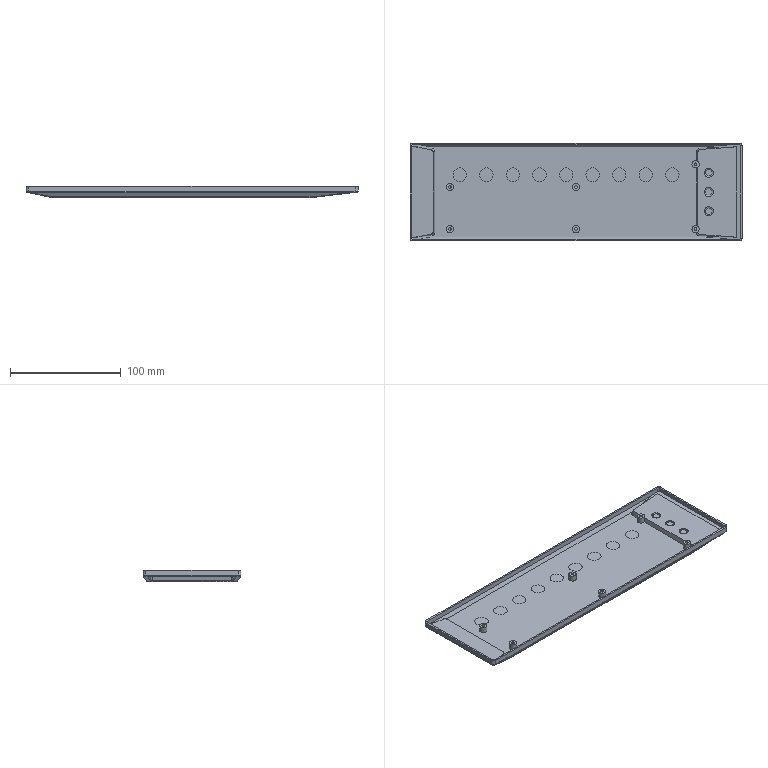NC program | NX | posted with a generic post | part box 300 x 88.5 x 10 mm
Lines 1165 to 2814 of 79950:
(CAVITY_MILL_COPY_COPY_1 , TOOL : D4)
N2322 T04 M6
N2324 G54
N2326 G17 G0 G90 X-96.335 Y33.695 S9500 M3
N2328 G43 Z30. H4
N2330 Z0.8
N2332 G94 G1 Z-0.2 F1000.
N2334 X-96.706 Y34.138
N2336 G3 X-97.473 Y34.495 R1.
N2338 G1 X-98.111 F1650.
N2340 X-98.634 Y34.128
N2342 G3 X-99.055 Y33.396 R1.
N2344 G1 X-99.105 Y32.82
N2346 Z0.8
N2348 G0 X-95.766 Y31.895 Z0.5
N2350 G1 Z-0.5 F1000.
N2352 X-96.138 Y32.338
N2354 G3 X-96.904 Y32.695 R1.
N2356 G1 X-97.542 F1650.
N2358 X-98.065 Y32.328
N2360 G3 X-98.486 Y31.596 R1.
N2362 G1 X-98.536 Y31.02
N2364 Z0.5
N2366 G0 X-95.752 Y31.85 Z0.25
N2368 G1 Z-0.75 F1000.
N2370 X-96.123 Y32.293
N2372 G3 X-96.889 Y32.65 R1.
N2374 G1 X-97.528 F1650.
N2376 X-98.051 Y32.283
N2378 G3 X-98.472 Y31.551 R1.
N2380 G1 X-98.522 Y30.975
N2382 Z0.25
N2384 G0 X-95.752 Y31.85 Z0.
N2386 G1 Z-1. F1000.
N2388 X-96.123 Y32.293
N2390 G3 X-96.889 Y32.65 R1.
N2392 G1 X-97.528 F1650.
N2394 X-98.051 Y32.283
N2396 G3 X-98.472 Y31.551 R1.
N2398 G1 X-98.522 Y30.975
N2400 Z0.
N2402 G0 Z30.
N2404 X-113.253 Y33.33
N2406 Z0.5
N2408 G1 Z-0.5 F1000.
N2410 X-112.81 Y33.702
N2412 G3 X-112.453 Y34.468 R1.
N2414 G1 Y35.999 F1650.
N2416 X-112.732 Y36.02
N2418 G2 X-113.655 Y36.323 R2.
N2420 G3 X-114.493 Y36.429 R1.
N2422 G1 X-114.82 Y36.324
N2424 Z0.5
N2426 G0 X-113.322 Y32.93 Z0.25
N2428 G1 Z-0.75 F1000.
N2430 X-112.879 Y33.302
N2432 G3 X-112.522 Y34.068 R1.
N2434 G1 Y35.935 F1650.
N2436 X-114.384 Y36.07
N2438 G3 X-115.174 Y35.769 R1.
N2440 G1 X-115.518 Y35.414
N2442 Z0.25
N2444 G0 X-113.387 Y32.87 Z0.
N2446 G1 Z-1. F1000.
N2448 X-112.944 Y33.242
N2450 G3 X-112.587 Y34.008 R1.
N2452 G1 Y35.875 F1650.
N2454 X-114.449 Y36.009
N2456 G3 X-115.239 Y35.708 R1.
N2458 G1 X-115.641 Y35.293
N2460 Z0.
N2462 G0 X-113.49 Y32.774 Z-0.378
N2464 G1 Z-1.378 F1000.
N2466 X-113.047 Y33.146
N2468 G3 X-112.69 Y33.912 R1.
N2470 G1 Y35.779 F1650.
N2472 X-114.552 Y35.913
N2474 G3 X-115.342 Y35.612 R1.
N2476 G1 X-115.745 Y35.197
N2478 Z-0.378
N2480 G0 X-113.591 Y32.68 Z-0.756
N2482 G1 Z-1.756 F1000.
N2484 X-113.149 Y33.051
N2486 G3 X-112.791 Y33.817 R1.
N2488 G1 Y35.684 F1650.
N2490 X-114.654 Y35.819
N2492 G3 X-115.443 Y35.518 R1.
N2494 G1 X-115.846 Y35.103
N2496 Z-0.756
N2498 G0 X-113.693 Y32.586 Z-1.133
N2500 G1 Z-2.133 F1000.
N2502 X-113.25 Y32.957
N2504 G3 X-112.893 Y33.723 R1.
N2506 G1 Y35.59 F1650.
N2508 X-114.755 Y35.725
N2510 G3 X-115.545 Y35.424 R1.
N2512 G1 X-115.947 Y35.009
N2514 Z-1.133
N2516 G0 X-113.794 Y32.491 Z-1.511
N2518 G1 Z-2.511 F1000.
N2520 X-113.351 Y32.863
N2522 G3 X-112.994 Y33.629 R1.
N2524 G1 Y35.496 F1650.
N2526 X-114.856 Y35.631
N2528 G3 X-115.646 Y35.33 R1.
N2530 G1 X-116.048 Y34.915
N2532 Z-1.511
N2534 G0 X-113.895 Y32.397 Z-1.889
N2536 G1 Z-2.889 F1000.
N2538 X-113.452 Y32.769
N2540 G3 X-113.095 Y33.535 R1.
N2542 G1 Y35.402 F1650.
N2544 X-114.957 Y35.537
N2546 G3 X-115.747 Y35.236 R1.
N2548 G1 X-116.15 Y34.821
N2550 Z-1.889
N2552 G0 X-113.996 Y32.303 Z-2.267
N2554 G1 Z-3.267 F1000.
N2556 X-113.554 Y32.675
N2558 G3 X-113.196 Y33.441 R1.
N2560 G1 Y35.308 F1650.
N2562 X-115.059 Y35.442
N2564 G3 X-115.848 Y35.141 R1.
N2566 G1 X-116.251 Y34.727
N2568 Z-2.267
N2570 G0 X-114.098 Y32.209 Z-2.644
N2572 G1 Z-3.644 F1000.
N2574 X-113.655 Y32.581
N2576 G3 X-113.298 Y33.347 R1.
N2578 G1 Y35.214 F1650.
N2580 X-115.16 Y35.348
N2582 G3 X-115.95 Y35.047 R1.
N2584 G1 X-116.352 Y34.632
N2586 Z-2.644
N2588 G0 X-114.199 Y32.115 Z-3.022
N2590 G1 Z-4.022 F1000.
N2592 X-113.756 Y32.486
N2594 G3 X-113.399 Y33.252 R1.
N2596 G1 Y35.119 F1650.
N2598 X-115.261 Y35.254
N2600 G3 X-116.051 Y34.953 R1.
N2602 G1 X-116.453 Y34.538
N2604 Z-3.022
N2606 G0 X-114.298 Y32.022 Z-3.4
N2608 G1 Z-4.4 F1000.
N2610 X-113.855 Y32.394
N2612 G3 X-113.498 Y33.16 R1.
N2614 G1 Y35.027 F1650.
N2616 X-115.36 Y35.162
N2618 G3 X-116.15 Y34.861 R1.
N2620 G1 X-116.553 Y34.446
N2622 Z-3.4
N2624 G0 Z30.
N2626 X-100.598 Y31.771
N2628 Z0.8
N2630 G1 Z-0.2 F1000.
N2632 X-101.157 Y31.92
N2634 G3 X-101.989 Y31.772 R1.
N2636 G1 X-102.845 Y31.171 F1650.
N2638 Y30.125
N2640 G3 X-102.488 Y29.359 R1.
N2642 G1 X-102.045 Y28.987
N2644 Z0.8
N2646 G0 X-98.798 Y30.835 Z0.5
N2648 G1 Z-0.5 F1000.
N2650 X-99.357 Y30.984
N2652 G3 X-100.189 Y30.836 R1.
N2654 G1 X-101.045 Y30.235 F1650.
N2656 Y29.189
N2658 G3 X-100.688 Y28.423 R1.
N2660 G1 X-100.245 Y28.052
N2662 Z0.5
N2664 G0 X-98.753 Y30.812 Z0.25
N2666 G1 Z-0.75 F1000.
N2668 X-99.312 Y30.961
N2670 G3 X-100.144 Y30.813 R1.
N2672 G1 X-101. Y30.212 F1650.
N2674 Y29.166
N2676 G3 X-100.643 Y28.4 R1.
N2678 G1 X-100.2 Y28.028
N2680 Z0.25
N2682 G0 X-98.753 Y30.812 Z0.
N2684 G1 Z-1. F1000.
N2686 X-99.312 Y30.961
N2688 G3 X-100.144 Y30.813 R1.
N2690 G1 X-101. Y30.212 F1650.
N2692 Y29.166
N2694 G3 X-100.643 Y28.4 R1.
N2696 G1 X-100.2 Y28.028
N2698 Z0.
N2700 G0 Z30.
N2702 X-118.722 Y18.574
N2704 Z-2.9
N2706 G1 X-118.754 Y18.627 Z-2.903 F1000.
N2708 X-119.176 Y18.964 Z-2.932
N2710 X-119.684 Y19.15 Z-2.96
N2712 X-120.003 Z-2.977
N2714 X-120.319 Z-2.993
N2716 X-120.825 Y18.964 Z-3.021
N2718 X-121.246 Y18.627 Z-3.05
N2720 X-121.574 Y18.086 Z-3.083
N2722 X-121.675 Y17.37 Z-3.121
N2724 X-121.465 Y16.677 Z-3.159
N2726 X-120.983 Y16.138 Z-3.197
N2728 X-120.319 Y15.85 Z-3.235
N2730 X-119.686 Z-3.268
N2732 X-119.02 Y16.135 Z-3.306
N2734 X-118.536 Y16.675 Z-3.344
N2736 X-118.325 Y17.369 Z-3.382
N2738 X-118.426 Y18.086 Z-3.42
N2740 X-118.754 Y18.627 Z-3.453
N2742 X-119.176 Y18.964 Z-3.481
N2744 X-119.684 Y19.15 Z-3.509
N2746 X-120.003 Z-3.526
N2748 X-120.319 Z-3.543
N2750 X-120.825 Y18.964 Z-3.571
N2752 X-121.246 Y18.627 Z-3.599
N2754 X-121.574 Y18.086 Z-3.632
N2756 X-121.675 Y17.37 Z-3.67
N2758 X-121.465 Y16.677 Z-3.708
N2760 X-120.983 Y16.138 Z-3.746
N2762 X-120.319 Y15.85 Z-3.784
N2764 X-119.686 Z-3.817
N2766 X-119.02 Y16.135 Z-3.855
N2768 X-118.536 Y16.675 Z-3.893
N2770 X-118.325 Y17.369 Z-3.931
N2772 X-118.426 Y18.086 Z-3.969
N2774 X-118.754 Y18.627 Z-4.002
N2776 X-119.176 Y18.964 Z-4.031
N2778 X-119.684 Y19.15 Z-4.059
N2780 X-120.003 Z-4.076
N2782 X-120.319 Z-4.092
N2784 X-120.825 Y18.964 Z-4.12
N2786 X-121.246 Y18.627 Z-4.149
N2788 X-121.574 Y18.086 Z-4.182
N2790 X-121.675 Y17.37 Z-4.22
N2792 X-121.465 Y16.677 Z-4.258
N2794 X-120.983 Y16.138 Z-4.296
N2796 X-120.319 Y15.85 Z-4.334
N2798 X-119.686 Z-4.367
N2800 X-119.02 Y16.135 Z-4.405
N2802 X-118.536 Y16.675 Z-4.443
N2804 X-118.325 Y17.369 Z-4.481
N2806 X-118.426 Y18.086 Z-4.519
N2808 X-118.754 Y18.627 Z-4.552
N2810 X-119.176 Y18.964 Z-4.58
N2812 X-119.684 Y19.15 Z-4.608
N2814 X-120. Z-4.625
N2816 X-120.003 F1650.
N2818 G3 X-121.65 Y17.498 R1.65
N2820 X-120. Y19.15 R-1.65
N2822 X-120.766 Y18.793 R1.
N2824 G1 Z-3.625
N2826 G0 Z30.
N2828 X-121.121 Y17.493
N2830 Z-3.125
N2832 G1 X-121.062 Y17.072 Z-3.147 F1000.
N2834 X-120.737 Y16.623 Z-3.176
N2836 X-120.239 Y16.38 Z-3.205
N2838 X-119.718 Y16.39 Z-3.233
N2840 X-119.241 Y16.643 Z-3.261
N2842 X-118.932 Y17.086 Z-3.289
N2844 X-118.861 Y17.621 Z-3.318
N2846 X-119.033 Y18.113 Z-3.345
N2848 X-119.337 Y18.433 Z-3.368
N2850 X-119.74 Y18.615 Z-3.391
N2852 X-120.002 Z-3.405
N2854 X-120.263 Y18.614 Z-3.419
N2856 X-120.664 Y18.433 Z-3.442
N2858 X-120.967 Y18.113 Z-3.465
N2860 X-121.139 Y17.621 Z-3.492
N2862 X-121.062 Y17.072 Z-3.521
N2864 X-120.737 Y16.623 Z-3.55
N2866 X-120.239 Y16.38 Z-3.579
N2868 X-119.718 Y16.39 Z-3.606
N2870 X-119.241 Y16.643 Z-3.635
N2872 X-118.932 Y17.086 Z-3.663
N2874 X-118.861 Y17.621 Z-3.691
N2876 X-119.033 Y18.113 Z-3.719
N2878 X-119.337 Y18.433 Z-3.742
N2880 X-119.74 Y18.615 Z-3.765
N2882 X-120.002 Z-3.779
N2884 X-120.263 Y18.614 Z-3.792
N2886 X-120.664 Y18.433 Z-3.815
N2888 X-120.967 Y18.113 Z-3.839
N2890 X-121.139 Y17.621 Z-3.866
N2892 X-121.062 Y17.072 Z-3.895
N2894 X-120.737 Y16.623 Z-3.924
N2896 X-120.239 Y16.38 Z-3.953
N2898 X-119.718 Y16.39 Z-3.98
N2900 X-119.241 Y16.643 Z-4.009
N2902 X-118.932 Y17.086 Z-4.037
N2904 X-118.861 Y17.621 Z-4.065
N2906 X-119.033 Y18.113 Z-4.092
N2908 X-119.337 Y18.433 Z-4.116
N2910 X-119.74 Y18.615 Z-4.139
N2912 X-120.002 Z-4.153
N2914 X-120.263 Y18.614 Z-4.166
N2916 X-120.664 Y18.433 Z-4.189
N2918 X-120.967 Y18.113 Z-4.212
N2920 X-121.139 Y17.621 Z-4.24
N2922 X-121.062 Y17.072 Z-4.269
N2924 X-120.737 Y16.623 Z-4.298
N2926 X-120.239 Y16.38 Z-4.327
N2928 X-119.718 Y16.39 Z-4.354
N2930 X-119.241 Y16.643 Z-4.382
N2932 X-118.932 Y17.086 Z-4.411
N2934 X-118.861 Y17.621 Z-4.439
N2936 X-119.033 Y18.113 Z-4.466
N2938 X-119.337 Y18.433 Z-4.489
N2940 X-119.74 Y18.615 Z-4.513
N2942 X-120.002 Z-4.526
N2944 X-120.263 Y18.614 Z-4.54
N2946 X-120.664 Y18.433 Z-4.563
N2948 X-120.967 Y18.113 Z-4.586
N2950 X-121.139 Y17.621 Z-4.613
N2952 X-121.062 Y17.072 Z-4.642
N2954 X-120.737 Y16.623 Z-4.672
N2956 X-120.239 Y16.38 Z-4.701
N2958 X-119.718 Y16.39 Z-4.728
N2960 X-119.241 Y16.643 Z-4.756
N2962 X-118.932 Y17.086 Z-4.784
N2964 X-118.861 Y17.621 Z-4.813
N2966 X-119.033 Y18.113 Z-4.84
N2968 X-119.337 Y18.433 Z-4.863
N2970 X-119.74 Y18.615 Z-4.886
N2972 X-120. Z-4.9
N2974 X-120.002 F1650.
N2976 G3 X-121.115 Y17.498 R1.115
N2978 X-120. Y18.615 R-1.115
N2980 X-120.766 Y18.258 R1.
N2982 G1 Z-3.9
N2984 G0 Z30.
N2986 X-121.073 Y1.258
N2988 Z-2.9
N2990 G1 X-121.337 Y1.017 Z-2.919 F1000.
N2992 X-121.618 Y0.451 Z-2.952
N2994 X-121.65 Y0.316 Z-2.959
N2996 Y-0.316 Z-2.992
N2998 X-121.4 Y-0.929 Z-3.027
N3000 X-120.931 Y-1.398 Z-3.062
N3002 X-120.319 Y-1.65 Z-3.096
N3004 X-119.686 Z-3.13
N3006 X-119.049 Y-1.385 Z-3.166
N3008 X-118.573 Y-0.886 Z-3.202
N3010 X-118.337 Y-0.237 Z-3.238
N3012 X-118.382 Y0.451 Z-3.274
N3014 X-118.663 Y1.017 Z-3.307
N3016 X-119.116 Y1.429 Z-3.339
N3018 X-119.686 Y1.65 Z-3.371
N3020 X-120.319 Z-3.405
N3022 X-120.886 Y1.427 Z-3.437
N3024 X-121.337 Y1.017 Z-3.468
N3026 X-121.618 Y0.451 Z-3.502
N3028 X-121.65 Y0.316 Z-3.509
N3030 Y-0.316 Z-3.542
N3032 X-121.4 Y-0.929 Z-3.577
N3034 X-120.931 Y-1.398 Z-3.611
N3036 X-120.319 Y-1.65 Z-3.646
N3038 X-119.686 Z-3.679
N3040 X-119.049 Y-1.385 Z-3.715
N3042 X-118.573 Y-0.886 Z-3.752
N3044 X-118.337 Y-0.237 Z-3.788
N3046 X-118.382 Y0.451 Z-3.824
N3048 X-118.663 Y1.017 Z-3.857
N3050 X-119.116 Y1.429 Z-3.889
N3052 X-119.686 Y1.65 Z-3.921
N3054 X-120.319 Z-3.954
N3056 X-120.886 Y1.427 Z-3.986
N3058 X-121.337 Y1.017 Z-4.018
N3060 X-121.618 Y0.451 Z-4.051
N3062 X-121.65 Y0.316 Z-4.059
N3064 Y-0.316 Z-4.092
N3066 X-121.4 Y-0.929 Z-4.127
N3068 X-120.931 Y-1.398 Z-4.161
N3070 X-120.319 Y-1.65 Z-4.196
N3072 X-119.686 Z-4.229
N3074 X-119.049 Y-1.385 Z-4.265
N3076 X-118.573 Y-0.886 Z-4.301
N3078 X-118.337 Y-0.237 Z-4.338
N3080 X-118.382 Y0.451 Z-4.374
N3082 X-118.663 Y1.017 Z-4.407
N3084 X-119.116 Y1.429 Z-4.439
N3086 X-119.686 Y1.65 Z-4.471
N3088 X-120.319 Z-4.504
N3090 X-120.886 Y1.427 Z-4.536
N3092 X-121.337 Y1.017 Z-4.568
N3094 X-121.618 Y0.451 Z-4.601
N3096 X-121.65 Y0.316 Z-4.608
N3098 Y0. Z-4.625
N3100 G3 X-120. Y-1.65 R1.65 F1650.
N3102 X-121.65 Y0. R-1.65
N3104 X-121.293 Y-0.766 R1.
N3106 G1 Z-3.625
N3108 G0 Z30.
N3110 X-120.024 Y-1.115
N3112 Z-3.125
N3114 G1 X-119.742 Y-1.116 Z-3.14 F1000.
N3116 X-119.287 Y-0.896 Z-3.166
N3118 X-118.971 Y-0.501 Z-3.193
N3120 X-118.855 Y-0.009 Z-3.219
N3122 X-118.969 Y0.499 Z-3.247
N3124 X-119.286 Y0.895 Z-3.273
N3126 X-119.742 Y1.116 Z-3.3
N3128 X-120.263 Y1.114 Z-3.327
N3130 X-120.716 Y0.893 Z-3.353
N3132 X-121.031 Y0.499 Z-3.38
N3134 X-121.115 Y0.124 Z-3.4
N3136 Y-0.26 Z-3.42
N3138 X-120.81 Y-0.809 Z-3.453
N3140 X-120.263 Y-1.114 Z-3.486
N3142 X-119.742 Y-1.116 Z-3.513
N3144 X-119.287 Y-0.896 Z-3.54
N3146 X-118.971 Y-0.501 Z-3.566
N3148 X-118.855 Y-0.009 Z-3.593
N3150 X-118.969 Y0.499 Z-3.62
N3152 X-119.286 Y0.895 Z-3.646
N3154 X-119.742 Y1.116 Z-3.673
N3156 X-120.263 Y1.114 Z-3.7
N3158 X-120.716 Y0.893 Z-3.727
N3160 X-121.031 Y0.499 Z-3.753
N3162 X-121.115 Y0.124 Z-3.773
N3164 Y-0.26 Z-3.793
N3166 X-120.81 Y-0.809 Z-3.826
N3168 X-120.263 Y-1.114 Z-3.859
N3170 X-119.742 Y-1.116 Z-3.887
N3172 X-119.287 Y-0.896 Z-3.913
N3174 X-118.971 Y-0.501 Z-3.94
N3176 X-118.855 Y-0.009 Z-3.966
N3178 X-118.969 Y0.499 Z-3.993
N3180 X-119.286 Y0.895 Z-4.02
N3182 X-119.742 Y1.116 Z-4.046
N3184 X-120.263 Y1.114 Z-4.074
N3186 X-120.716 Y0.893 Z-4.1
N3188 X-121.031 Y0.499 Z-4.127
N3190 X-121.115 Y0.124 Z-4.147
N3192 Y-0.26 Z-4.167
N3194 X-120.81 Y-0.809 Z-4.2
N3196 X-120.263 Y-1.114 Z-4.233
N3198 X-119.742 Y-1.116 Z-4.26
N3200 X-119.287 Y-0.896 Z-4.286
N3202 X-118.971 Y-0.501 Z-4.313
N3204 X-118.855 Y-0.009 Z-4.339
N3206 X-118.969 Y0.499 Z-4.367
N3208 X-119.286 Y0.895 Z-4.393
N3210 X-119.742 Y1.116 Z-4.42
N3212 X-120.263 Y1.114 Z-4.447
N3214 X-120.716 Y0.893 Z-4.474
N3216 X-121.031 Y0.499 Z-4.5
N3218 X-121.115 Y0.124 Z-4.52
N3220 Y-0.26 Z-4.54
N3222 X-120.81 Y-0.809 Z-4.573
N3224 X-120.263 Y-1.114 Z-4.606
N3226 X-119.742 Y-1.116 Z-4.633
N3228 X-119.287 Y-0.896 Z-4.66
N3230 X-118.971 Y-0.501 Z-4.686
N3232 X-118.855 Y-0.009 Z-4.713
N3234 X-118.969 Y0.499 Z-4.74
N3236 X-119.286 Y0.895 Z-4.767
N3238 X-119.742 Y1.116 Z-4.793
N3240 X-120.263 Y1.114 Z-4.82
N3242 X-120.716 Y0.893 Z-4.847
N3244 X-121.031 Y0.499 Z-4.873
N3246 X-121.115 Y0.124 Z-4.894
N3248 Y0. Z-4.9
N3250 G3 X-120. Y-1.115 R1.115 F1650.
N3252 X-121.115 Y0. R-1.115
N3254 X-120.758 Y-0.766 R1.
N3256 G1 Z-3.9
N3258 G0 Z30.
N3260 X-102.045 Y5.626
N3262 Z0.8
N3264 G1 Z-0.2 F1000.
N3266 X-102.488 Y5.255
N3268 G3 X-102.845 Y4.489 R1.
N3270 G1 Y3.507 F1650.
N3272 X-102.071 Y2.902
N3274 G3 X-101.248 Y2.712 R1.
N3276 G1 X-100.682 Y2.833
N3278 Z0.8
N3280 G0 X-100.245 Y6.504 Z0.5
N3282 G1 Z-0.5 F1000.
N3284 X-100.688 Y6.133
N3286 G3 X-101.045 Y5.367 R1.
N3288 G1 Y4.385 F1650.
N3290 X-100.271 Y3.78
N3292 G3 X-99.448 Y3.59 R1.
N3294 G1 X-98.882 Y3.71
N3296 Z0.5
N3298 G0 X-100.2 Y6.526 Z0.25
N3300 G1 Z-0.75 F1000.
N3302 X-100.643 Y6.155
N3304 G3 X-101. Y5.389 R1.
N3306 G1 Y4.407 F1650.
N3308 X-100.226 Y3.802
N3310 G3 X-99.403 Y3.612 R1.
N3312 G1 X-98.837 Y3.732
N3314 Z0.25
N3316 G0 X-100.2 Y6.526 Z0.
N3318 G1 Z-1. F1000.
N3320 X-100.643 Y6.155
N3322 G3 X-101. Y5.389 R1.
N3324 G1 Y4.407 F1650.
N3326 X-100.226 Y3.802
N3328 G3 X-99.403 Y3.612 R1.
N3330 G1 X-98.837 Y3.732
N3332 Z0.
N3334 G0 Z30.
N3336 X-112.898 Y-9.686
N3338 Z0.8
N3340 G1 Z-0.2 F1000.
N3342 X-112.534 Y-9.453
N3344 G3 X-112.081 Y-8.74 R1.
N3346 G2 X-111.655 Y-7.753 R1.953 F1650.
N3348 X-112.058 Y-6.885 R2.04
N3350 G3 X-112.559 Y-6.204 R1.
N3352 G1 X-112.898 Y-6.019
N3354 Z0.8
N3356 G0 Z30.
N3358 Y-19.477
N3360 Z0.8
N3362 G1 Z-0.2 F1000.
N3364 X-112.553 Y-19.29
N3366 G3 X-112.05 Y-18.611 R1.
N3368 G2 X-111.702 Y-17.757 R2.489 F1650.
N3370 X-112.073 Y-16.751 R2.599
N3372 G3 X-112.538 Y-16.045 R1.
N3374 G1 X-112.898 Y-15.823
N3376 Z0.8
N3378 G0 Z30.
N3380 Y-29.706
N3382 Z0.8
N3384 G1 Z-0.2 F1000.
N3386 X-112.539 Y-29.486
N3388 G3 X-112.073 Y-28.781 R1.
N3390 G2 X-111.696 Y-27.701 R3.057 F1650.
N3392 X-112.058 Y-26.885 R2.034
N3394 G3 X-112.559 Y-26.204 R1.
N3396 G1 X-112.898 Y-26.018
N3398 Z0.8
N3400 G0 Z30.
N3402 Y-39.479
N3404 Z0.8
N3406 G1 Z-0.2 F1000.
N3408 X-112.554 Y-39.293
N3410 G3 X-112.052 Y-38.614 R1.
N3412 G2 X-111.688 Y-37.752 R2.371 F1650.
N3414 X-112.074 Y-36.774 R2.318
N3416 G3 X-112.539 Y-36.068 R1.
N3418 G1 X-112.898 Y-35.847
N3420 Z0.8
N3422 G0 X-114.837 Y-36.368 Z0.5
N3424 G1 Z-0.5 F1000.
N3426 X-114.505 Y-36.468
N3428 G3 X-113.669 Y-36.346 R1.
N3430 G2 X-112.662 Y-36.014 R2.038 F1650.
N3432 G1 X-112.453 Y-35.999
N3434 Y-34.468
N3436 G3 X-112.81 Y-33.702 R1.
N3438 G1 X-113.253 Y-33.33
N3440 Z0.5
N3442 G0 X-115.518 Y-35.414 Z0.25
N3444 G1 Z-0.75 F1000.
N3446 X-115.174 Y-35.769
N3448 G3 X-114.384 Y-36.07 R1.
N3450 G1 X-112.522 Y-35.935 F1650.
N3452 Y-34.068
N3454 G3 X-112.879 Y-33.302 R1.
N3456 G1 X-113.322 Y-32.93
N3458 Z0.25
N3460 G0 X-115.641 Y-35.293 Z0.
N3462 G1 Z-1. F1000.
N3464 X-115.239 Y-35.708
N3466 G3 X-114.449 Y-36.009 R1.
N3468 G1 X-112.587 Y-35.875 F1650.
N3470 Y-34.008
N3472 G3 X-112.944 Y-33.242 R1.
N3474 G1 X-113.387 Y-32.87
N3476 Z0.
N3478 G0 X-115.745 Y-35.197 Z-0.378
N3480 G1 Z-1.378 F1000.
N3482 X-115.342 Y-35.612
N3484 G3 X-114.552 Y-35.913 R1.
N3486 G1 X-112.69 Y-35.779 F1650.
N3488 Y-33.912
N3490 G3 X-113.047 Y-33.146 R1.
N3492 G1 X-113.49 Y-32.774
N3494 Z-0.378
N3496 G0 X-115.846 Y-35.103 Z-0.756
N3498 G1 Z-1.756 F1000.
N3500 X-115.443 Y-35.518
N3502 G3 X-114.654 Y-35.819 R1.
N3504 G1 X-112.791 Y-35.684 F1650.
N3506 Y-33.817
N3508 G3 X-113.149 Y-33.051 R1.
N3510 G1 X-113.591 Y-32.68
N3512 Z-0.756
N3514 G0 X-115.947 Y-35.009 Z-1.133
N3516 G1 Z-2.133 F1000.
N3518 X-115.545 Y-35.424
N3520 G3 X-114.755 Y-35.725 R1.
N3522 G1 X-112.893 Y-35.59 F1650.
N3524 Y-33.723
N3526 G3 X-113.25 Y-32.957 R1.
N3528 G1 X-113.693 Y-32.586
N3530 Z-1.133
N3532 G0 X-116.048 Y-34.915 Z-1.511
N3534 G1 Z-2.511 F1000.
N3536 X-115.646 Y-35.33
N3538 G3 X-114.856 Y-35.631 R1.
N3540 G1 X-112.994 Y-35.496 F1650.
N3542 Y-33.629
N3544 G3 X-113.351 Y-32.863 R1.
N3546 G1 X-113.794 Y-32.491
N3548 Z-1.511
N3550 G0 X-116.15 Y-34.821 Z-1.889
N3552 G1 Z-2.889 F1000.
N3554 X-115.747 Y-35.236
N3556 G3 X-114.957 Y-35.537 R1.
N3558 G1 X-113.095 Y-35.402 F1650.
N3560 Y-33.535
N3562 G3 X-113.452 Y-32.769 R1.
N3564 G1 X-113.895 Y-32.397
N3566 Z-1.889
N3568 G0 X-116.251 Y-34.727 Z-2.267
N3570 G1 Z-3.267 F1000.
N3572 X-115.848 Y-35.141
N3574 G3 X-115.059 Y-35.442 R1.
N3576 G1 X-113.196 Y-35.308 F1650.
N3578 Y-33.441
N3580 G3 X-113.554 Y-32.675 R1.
N3582 G1 X-113.996 Y-32.303
N3584 Z-2.267
N3586 G0 X-116.352 Y-34.632 Z-2.644
N3588 G1 Z-3.644 F1000.
N3590 X-115.95 Y-35.047
N3592 G3 X-115.16 Y-35.348 R1.
N3594 G1 X-113.298 Y-35.214 F1650.
N3596 Y-33.347
N3598 G3 X-113.655 Y-32.581 R1.
N3600 G1 X-114.098 Y-32.209
N3602 Z-2.644
N3604 G0 X-116.453 Y-34.538 Z-3.022
N3606 G1 Z-4.022 F1000.
N3608 X-116.051 Y-34.953
N3610 G3 X-115.261 Y-35.254 R1.
N3612 G1 X-113.399 Y-35.119 F1650.
N3614 Y-33.252
N3616 G3 X-113.756 Y-32.486 R1.
N3618 G1 X-114.199 Y-32.115
N3620 Z-3.022
N3622 G0 X-116.553 Y-34.446 Z-3.4
N3624 G1 Z-4.4 F1000.
N3626 X-116.15 Y-34.861
N3628 G3 X-115.36 Y-35.162 R1.
N3630 G1 X-113.498 Y-35.027 F1650.
N3632 Y-33.16
N3634 G3 X-113.855 Y-32.394 R1.
N3636 G1 X-114.298 Y-32.022
N3638 Z-3.4
N3640 G0 Z30.
N3642 X-112.898 Y-34.505
N3644 Z0.8
N3646 G1 Z-0.2 F1000.
N3648 X-112.553 Y-34.313
N3650 G3 X-112.057 Y-33.628 R1.
N3652 G2 X-111.687 Y-32.749 R2.299 F1650.
N3654 X-112.069 Y-31.79 R2.36
N3656 G3 X-112.544 Y-31.091 R1.
N3658 G1 X-112.898 Y-30.879
N3660 Z0.8
N3662 G0 Z30.
N3664 Y-24.346
N3666 Z0.8
N3668 G1 Z-0.2 F1000.
N3670 X-112.569 Y-24.185
N3672 G3 X-112.039 Y-23.526 R1.
N3674 G2 X-111.668 Y-22.762 R2.022 F1650.
N3676 X-112.035 Y-21.984 R2.179
N3678 G3 X-112.565 Y-21.325 R1.
N3680 G1 X-112.898 Y-21.162
N3682 Z0.8
N3684 G0 Z30.
N3686 X-121.292 Y-18.486
N3688 Z-2.9
N3690 G1 X-121.101 Y-18.769 Z-2.918 F1000.
N3692 X-120.319 Y-19.15 Z-2.963
N3694 X-120. Z-2.98
N3696 X-119.684 Z-2.997
N3698 X-118.901 Y-18.77 Z-3.042
N3700 X-118.412 Y-18.05 Z-3.088
N3702 X-118.35 Y-17.181 Z-3.134
N3704 X-118.585 Y-16.594 Z-3.167
N3706 X-119.059 Y-16.108 Z-3.202
N3708 X-119.686 Y-15.85 Z-3.238
N3710 X-120.319 Z-3.271
N3712 X-120.943 Y-16.11 Z-3.306
N3714 X-121.415 Y-16.594 Z-3.342
N3716 X-121.65 Y-17.181 Z-3.375
N3718 X-121.588 Y-18.049 Z-3.421
N3720 X-121.101 Y-18.769 Z-3.466
N3722 X-120.319 Y-19.15 Z-3.512
N3724 X-120. Z-3.528
N3726 X-119.684 Z-3.545
N3728 X-118.901 Y-18.77 Z-3.591
N3730 X-118.412 Y-18.05 Z-3.636
N3732 X-118.35 Y-17.181 Z-3.682
N3734 X-118.585 Y-16.594 Z-3.715
N3736 X-119.059 Y-16.108 Z-3.751
N3738 X-119.686 Y-15.85 Z-3.786
N3740 X-120.319 Z-3.819
N3742 X-120.943 Y-16.11 Z-3.855
N3744 X-121.415 Y-16.594 Z-3.89
N3746 X-121.65 Y-17.181 Z-3.923
N3748 X-121.588 Y-18.049 Z-3.969
N3750 X-121.101 Y-18.769 Z-4.014
N3752 X-120.319 Y-19.15 Z-4.06
N3754 X-120. Z-4.077
N3756 X-119.684 Z-4.093
N3758 X-118.901 Y-18.77 Z-4.139
N3760 X-118.412 Y-18.05 Z-4.185
N3762 X-118.35 Y-17.181 Z-4.23
N3764 X-118.585 Y-16.594 Z-4.263
N3766 X-119.059 Y-16.108 Z-4.299
N3768 X-119.686 Y-15.85 Z-4.334
N3770 X-120.319 Z-4.368
N3772 X-120.943 Y-16.11 Z-4.403
N3774 X-121.415 Y-16.594 Z-4.438
N3776 X-121.65 Y-17.181 Z-4.472
N3778 X-121.588 Y-18.049 Z-4.517
N3780 X-121.101 Y-18.769 Z-4.563
N3782 X-120.319 Y-19.15 Z-4.608
N3784 X-120. Z-4.625
N3786 G3 X-118.35 Y-17.5 R1.65 F1650.
N3788 X-120. Y-19.15 R-1.65
N3790 X-119.234 Y-18.793 R1.
N3792 G1 Z-3.625
N3794 G0 Z30.
N3796 X-118.875 Y-17.565
N3798 Z-3.125
N3800 G1 X-118.925 Y-17.105 Z-3.149 F1000.
N3802 X-119.211 Y-16.67 Z-3.177
N3804 X-119.761 Y-16.38 Z-3.209
N3806 X-120.282 Y-16.39 Z-3.236
N3808 X-120.789 Y-16.67 Z-3.267
N3810 X-121.075 Y-17.105 Z-3.294
N3812 X-121.133 Y-17.663 Z-3.323
N3814 X-120.92 Y-18.181 Z-3.353
N3816 X-120.487 Y-18.536 Z-3.382
N3818 X-120.119 Y-18.615 Z-3.402
N3820 X-120. Z-3.408
N3822 X-119.869 Z-3.415
N3824 X-119.489 Y-18.525 Z-3.435
N3826 X-119.069 Y-18.167 Z-3.464
N3828 X-118.865 Y-17.654 Z-3.493
N3830 X-118.925 Y-17.105 Z-3.522
N3832 X-119.211 Y-16.67 Z-3.55
N3834 X-119.761 Y-16.38 Z-3.582
N3836 X-120.282 Y-16.39 Z-3.609
N3838 X-120.789 Y-16.67 Z-3.64
N3840 X-121.075 Y-17.105 Z-3.667
N3842 X-121.133 Y-17.663 Z-3.696
N3844 X-120.92 Y-18.181 Z-3.726
N3846 X-120.487 Y-18.536 Z-3.755
N3848 X-120.119 Y-18.615 Z-3.775
N3850 X-120. Z-3.781
N3852 X-119.869 Z-3.788
N3854 X-119.489 Y-18.525 Z-3.808
N3856 X-119.069 Y-18.167 Z-3.837
N3858 X-118.865 Y-17.654 Z-3.866
N3860 X-118.925 Y-17.105 Z-3.895
N3862 X-119.211 Y-16.67 Z-3.922
N3864 X-119.761 Y-16.38 Z-3.955
N3866 X-120.282 Y-16.39 Z-3.982
N3868 X-120.789 Y-16.67 Z-4.013
N3870 X-121.075 Y-17.105 Z-4.04
N3872 X-121.133 Y-17.663 Z-4.069
N3874 X-120.92 Y-18.181 Z-4.099
N3876 X-120.487 Y-18.536 Z-4.128
N3878 X-120.119 Y-18.615 Z-4.148
N3880 X-120. Z-4.154
N3882 X-119.869 Z-4.161
N3884 X-119.489 Y-18.525 Z-4.181
N3886 X-119.069 Y-18.167 Z-4.21
N3888 X-118.865 Y-17.654 Z-4.239
N3890 X-118.925 Y-17.105 Z-4.268
N3892 X-119.211 Y-16.67 Z-4.295
N3894 X-119.761 Y-16.38 Z-4.328
N3896 X-120.282 Y-16.39 Z-4.355
N3898 X-120.789 Y-16.67 Z-4.386
N3900 X-121.075 Y-17.105 Z-4.413
N3902 X-121.133 Y-17.663 Z-4.442
N3904 X-120.92 Y-18.181 Z-4.472
N3906 X-120.487 Y-18.536 Z-4.501
N3908 X-120.119 Y-18.615 Z-4.521
N3910 X-120. Z-4.527
N3912 X-119.869 Z-4.534
N3914 X-119.489 Y-18.525 Z-4.554
N3916 X-119.069 Y-18.167 Z-4.583
N3918 X-118.865 Y-17.654 Z-4.612
N3920 X-118.925 Y-17.105 Z-4.641
N3922 X-119.211 Y-16.67 Z-4.668
N3924 X-119.761 Y-16.38 Z-4.701
N3926 X-120.282 Y-16.39 Z-4.728
N3928 X-120.789 Y-16.67 Z-4.759
N3930 X-121.075 Y-17.105 Z-4.786
N3932 X-121.133 Y-17.663 Z-4.815
N3934 X-120.92 Y-18.181 Z-4.845
N3936 X-120.487 Y-18.536 Z-4.874
N3938 X-120.119 Y-18.615 Z-4.894
N3940 X-120. Z-4.9
N3942 G3 X-118.885 Y-17.5 R1.115 F1650.
N3944 X-120. Y-18.615 R-1.115
N3946 X-119.234 Y-18.258 R1.
N3948 G1 Z-3.9
N3950 G0 Z30.
N3952 X-112.898 Y-14.521
N3954 Z0.8
N3956 G1 Z-0.2 F1000.
N3958 X-112.555 Y-14.328
N3960 G3 X-112.063 Y-13.641 R1.
N3962 G2 X-111.683 Y-12.785 R2.041 F1650.
N3964 X-112.066 Y-11.792 R2.644
N3966 G3 X-112.544 Y-11.095 R1.
N3968 G1 X-112.898 Y-10.886
N3970 Z0.8
N3972 G0 Z30.
N3974 X-99.058 Y1.564
N3976 Z0.8
N3978 G1 Z-0.2 F1000.
N3980 X-99.038 Y0.986
N3982 G3 X-98.654 Y0.233 R1.
N3984 G1 X-98.107 Y-0.195 F1650.
N3986 X-97.412
N3988 G3 X-96.646 Y0.162 R1.
N3990 G1 X-96.274 Y0.605
N3992 Z0.8
N3994 G0 X-98.439 Y3.364 Z0.5
N3996 G1 Z-0.5 F1000.
N3998 X-98.418 Y2.786
N4000 G3 X-98.035 Y2.033 R1.
N4002 G1 X-97.487 Y1.605 F1650.
N4004 X-96.792
N4006 G3 X-96.026 Y1.962 R1.
N4008 G1 X-95.654 Y2.405
N4010 Z0.5
N4012 G0 X-98.423 Y3.409 Z0.25
N4014 G1 Z-0.75 F1000.
N4016 X-98.403 Y2.831
N4018 G3 X-98.019 Y2.078 R1.
N4020 G1 X-97.471 Y1.65 F1650.
N4022 X-96.776
N4024 G3 X-96.01 Y2.007 R1.
N4026 G1 X-95.639 Y2.45
N4028 Z0.25
N4030 G0 X-98.423 Y3.409 Z0.
N4032 G1 Z-1. F1000.
N4034 X-98.403 Y2.831
N4036 G3 X-98.019 Y2.078 R1.
N4038 G1 X-97.471 Y1.65 F1650.
N4040 X-96.776
N4042 G3 X-96.01 Y2.007 R1.
N4044 G1 X-95.639 Y2.45
N4046 Z0.
N4048 G0 Z30.
N4050 X-3.856 Y-23.8
N4052 Z0.8
N4054 G1 Z-0.2 F1000.
N4056 X-4.228 Y-23.357
N4058 G3 X-4.994 Y-23. R1.
N4060 G1 X-7. F1650.
N4062 Y-25.006
N4064 G3 X-6.643 Y-25.772 R1.
N4066 G1 X-6.2 Y-26.144
N4068 Z0.8
N4070 G0 X-3.856 Y-23.8 Z0.5
N4072 G1 Z-0.5 F1000.
N4074 X-4.228 Y-23.357
N4076 G3 X-4.994 Y-23. R1.
N4078 G1 X-7. F1650.
N4080 Y-25.006
N4082 G3 X-6.643 Y-25.772 R1.
N4084 G1 X-6.2 Y-26.144
N4086 Z0.5
N4088 G0 Z30.
N4090 Y-29.856
N4092 Z0.8
N4094 G1 Z-0.2 F1000.
N4096 X-6.643 Y-30.228
N4098 G3 X-7. Y-30.994 R1.
N4100 G1 Y-33. F1650.
N4102 X-4.994
N4104 G3 X-4.228 Y-32.643 R1.
N4106 G1 X-3.856 Y-32.2
N4108 Z0.8
N4110 G0 X-6.2 Y-29.856 Z0.5
N4112 G1 Z-0.5 F1000.
N4114 X-6.643 Y-30.228
N4116 G3 X-7. Y-30.994 R1.
N4118 G1 Y-33. F1650.
N4120 X-4.994
N4122 G3 X-4.228 Y-32.643 R1.
N4124 G1 X-3.856 Y-32.2
N4126 Z0.5
N4128 G0 Z30.
N4130 X96.2 Y-26.144
N4132 Z0.8
N4134 G1 Z-0.2 F1000.
N4136 X96.643 Y-25.772
N4138 G3 X97. Y-25.006 R1.
N4140 G1 Y-23. F1650.
N4142 X94.994
N4144 G3 X94.228 Y-23.357 R1.
N4146 G1 X93.856 Y-23.8
N4148 Z0.8
N4150 G0 X96.2 Y-26.144 Z0.5
N4152 G1 Z-0.5 F1000.
N4154 X96.643 Y-25.772
N4156 G3 X97. Y-25.006 R1.
N4158 G1 X96.999 Y-23. F1650.
N4160 X94.994
N4162 G3 X94.228 Y-23.357 R1.
N4164 G1 X93.856 Y-23.8
N4166 Z0.5
N4168 G0 Z30.
N4170 Y-32.2
N4172 Z0.8
N4174 G1 Z-0.2 F1000.
N4176 X94.228 Y-32.643
N4178 G3 X94.994 Y-33. R1.
N4180 G1 X97. F1650.
N4182 Y-30.994
N4184 G3 X96.643 Y-30.228 R1.
N4186 G1 X96.2 Y-29.856
N4188 Z0.8
N4190 G0 X93.856 Y-32.2 Z0.5
N4192 G1 Z-0.5 F1000.
N4194 X94.228 Y-32.643
N4196 G3 X94.994 Y-33. R1.
N4198 G1 X97. F1650.
N4200 Y-30.994
N4202 G3 X96.643 Y-30.228 R1.
N4204 G1 X96.2 Y-29.856
N4206 Z0.5
N4208 G0 Z30.
N4210 X130.205 Y-36.151
N4212 Z0.8
N4214 G1 Z-0.2 F1000.
N4216 X129.875 Y-36.313
N4218 G3 X129.346 Y-36.972 R1.
N4220 G2 X128.965 Y-37.751 R2.042 F1650.
N4222 X129.346 Y-38.525 R2.013
N4224 G3 X129.876 Y-39.183 R1.
N4226 G1 X130.205 Y-39.345
N4228 Z0.8
N4230 G0 Z30.
N4232 X132.201 Y-34.02
N4234 Z0.25
N4236 G1 Z-0.75 F1000.
N4238 X131.759 Y-34.391
N4240 G3 X131.401 Y-35.157 R1.
N4242 G1 Y-35.889 F1650.
N4244 G2 X131.807 Y-36.455 R2.125
N4246 G3 X132.466 Y-36.985 R1.
N4248 G1 X132.807 Y-37.069
N4250 Z0.25
N4252 G0 X132.266 Y-33.407 Z0.
N4254 G1 Z-1. F1000.
N4256 X131.824 Y-33.778
N4258 G3 X131.466 Y-34.545 R1.
N4260 G1 Y-35.833 F1650.
N4262 G2 X132.42 Y-36.256 R2.007
N4264 G3 X133.24 Y-36.46 R1.
N4266 G1 X133.578 Y-36.394
N4268 Z0.
N4270 G0 X132.37 Y-32.925 Z-0.378
N4272 G1 Z-1.378 F1000.
N4274 X131.927 Y-33.297
N4276 G3 X131.57 Y-34.063 R1.
N4278 G1 Y-35.747 F1650.
N4280 X133.229 Y-36.039
N4282 G3 X134.042 Y-35.809 R1.
N4284 G1 X134.306 Y-35.581
N4286 Z-0.378
N4288 G0 X132.471 Y-32.84 Z-0.756
N4290 G1 Z-1.756 F1000.
N4292 X132.028 Y-33.212
N4294 G3 X131.671 Y-33.978 R1.
N4296 G1 Y-35.662 F1650.
N4298 X133.33 Y-35.955
N4300 G3 X134.146 Y-35.736 R1.
N4302 G1 X134.589 Y-35.365
N4304 Z-0.756
N4306 G0 X132.572 Y-32.755 Z-1.133
N4308 G1 Z-2.133 F1000.
N4310 X132.129 Y-33.127
N4312 G3 X131.772 Y-33.893 R1.
N4314 G1 Y-35.577 F1650.
N4316 X133.431 Y-35.87
N4318 G3 X134.248 Y-35.651 R1.
N4320 G1 X134.69 Y-35.28
N4322 Z-1.133
N4324 G0 X132.673 Y-32.67 Z-1.511
N4326 G1 Z-2.511 F1000.
N4328 X132.231 Y-33.042
N4330 G3 X131.873 Y-33.808 R1.
N4332 G1 Y-35.492 F1650.
N4334 X133.532 Y-35.785
N4336 G3 X134.349 Y-35.566 R1.
N4338 G1 X134.792 Y-35.195
N4340 Z-1.511
N4342 G0 X132.775 Y-32.585 Z-1.889
N4344 G1 Z-2.889 F1000.
N4346 X132.332 Y-32.957
N4348 G3 X131.975 Y-33.723 R1.
N4350 G1 Y-35.408 F1650.
N4352 X133.634 Y-35.7
N4354 G3 X134.45 Y-35.481 R1.
N4356 G1 X134.893 Y-35.11
N4358 Z-1.889
N4360 G0 X132.876 Y-32.5 Z-2.267
N4362 G1 Z-3.267 F1000.
N4364 X132.433 Y-32.872
N4366 G3 X132.076 Y-33.638 R1.
N4368 G1 Y-35.323 F1650.
N4370 X133.735 Y-35.615
N4372 G3 X134.551 Y-35.396 R1.
N4374 G1 X134.994 Y-35.025
N4376 Z-2.267
N4378 G0 X132.977 Y-32.415 Z-2.644
N4380 G1 Z-3.644 F1000.
N4382 X132.534 Y-32.787
N4384 G3 X132.177 Y-33.553 R1.
N4386 G1 Y-35.238 F1650.
N4388 X133.836 Y-35.53
N4390 G3 X134.652 Y-35.311 R1.
N4392 G1 X135.095 Y-34.94
N4394 Z-2.644
N4396 G0 X133.078 Y-32.33 Z-3.022
N4398 G1 Z-4.022 F1000.
N4400 X132.635 Y-32.702
N4402 G3 X132.278 Y-33.468 R1.
N4404 G1 Y-35.153 F1650.
N4406 X133.937 Y-35.445
N4408 G3 X134.754 Y-35.226 R1.
N4410 G1 X135.196 Y-34.855
N4412 Z-3.022
N4414 G0 X133.177 Y-32.247 Z-3.4
N4416 G1 Z-4.4 F1000.
N4418 X132.735 Y-32.619
N4420 G3 X132.377 Y-33.385 R1.
N4422 G1 Y-35.069 F1650.
N4424 X134.036 Y-35.362
N4426 G3 X134.853 Y-35.143 R1.
N4428 G1 X135.296 Y-34.772
N4430 Z-3.4
N4432 G0 X133.24 Y-32.195 Z-3.625
N4434 G1 Z-4.625 F1000.
N4436 X132.797 Y-32.566
N4438 G3 X132.44 Y-33.333 R1.
N4440 G1 Y-35.017 F1650.
N4442 X134.099 Y-35.31
N4444 G3 X134.915 Y-35.091 R1.
N4446 G1 X135.358 Y-34.719
N4448 Z-3.625
N4450 G0 X133.298 Y-32.146 Z-3.85
N4452 G1 Z-4.85 F1000.
N4454 X132.855 Y-32.518
N4456 G3 X132.498 Y-33.284 R1.
N4458 G1 Y-34.968 F1650.
N4460 X134.157 Y-35.261
N4462 G3 X134.973 Y-35.042 R1.
N4464 G1 X135.416 Y-34.671
N4466 Z-3.85
N4468 G0 Z30.
N4470 X130.205 Y-30.957
N4472 Z0.8
N4474 G1 Z-0.2 F1000.
N4476 X129.855 Y-31.157
N4478 G3 X129.367 Y-31.848 R1.
N4480 G2 X129.02 Y-32.737 R2.482 F1650.
N4482 X129.371 Y-33.698 R2.791
N4484 G3 X129.85 Y-34.394 R1.
N4486 G1 X130.205 Y-34.604
N4488 Z0.8
N4490 G0 Z30.
N4492 Y-26.023
N4494 Z0.8
N4496 G1 Z-0.2 F1000.
N4498 X129.866 Y-26.209
N4500 G3 X129.366 Y-26.89 R1.
N4502 G2 X128.97 Y-27.744 R2.01 F1650.
N4504 X129.363 Y-28.604 R2.091
N4506 G3 X129.866 Y-29.283 R1.
N4508 G1 X130.205 Y-29.468
N4510 Z0.8
N4512 G0 Z30.
N4514 Y-21.152
N4516 Z0.8
N4518 G1 Z-0.2 F1000.
N4520 X129.877 Y-21.314
N4522 G3 X129.348 Y-21.974 R1.
N4524 G2 X128.965 Y-22.749 R1.984 F1650.
N4526 X129.347 Y-23.525 R2.02
N4528 G3 X129.876 Y-24.184 R1.
N4530 G1 X130.205 Y-24.346
N4532 Z0.8
N4534 G0 Z30.
N4536 Y-16.153
N4538 Z0.8
N4540 G1 Z-0.2 F1000.
N4542 X129.876 Y-16.315
N4544 G3 X129.346 Y-16.973 R1.
N4546 G2 X128.966 Y-17.75 R2.033 F1650.
N4548 X129.346 Y-18.528 R2.047
N4550 G3 X129.875 Y-19.187 R1.
N4552 G1 X130.205 Y-19.349
N4554 Z0.8
N4556 G0 Z30.
N4558 Y-11.141
N4560 Z0.8
N4562 G1 Z-0.2 F1000.
N4564 X129.875 Y-11.305
N4566 G3 X129.348 Y-11.966 R1.
N4568 G2 X128.964 Y-12.752 R2.037 F1650.
N4570 X129.348 Y-13.53 R2.005
N4572 G3 X129.876 Y-14.189 R1.
N4574 G1 X130.205 Y-14.351
N4576 Z0.8
N4578 G0 Z30.
N4580 Y-6.134
N4582 Z0.8
N4584 G1 Z-0.2 F1000.
N4586 X129.874 Y-6.299
N4588 G3 X129.348 Y-6.96 R1.
N4590 G2 X128.965 Y-7.75 R2.056 F1650.
N4592 X129.347 Y-8.531 R2.044
N4594 G3 X129.875 Y-9.191 R1.
N4596 G1 X130.205 Y-9.354
N4598 Z0.8
N4600 G0 Z30.
N4602 X114.7 Y0.605
N4604 Z0.8
N4606 G1 Z-0.2 F1000.
N4608 X115.072 Y0.162
N4610 G3 X115.838 Y-0.195 R1.
N4612 G1 X116.592 F1650.
N4614 X117.161 Y0.3
N4616 G3 X117.505 Y1.072 R1.
N4618 G1 X117.495 Y1.65
N4620 Z0.8
N4622 G0 X114.027 Y2.405 Z0.5
N4624 G1 Z-0.5 F1000.
N4626 X114.399 Y1.962
N4628 G3 X115.165 Y1.605 R1.
N4630 G1 X115.919 F1650.
N4632 X116.488 Y2.1
N4634 G3 X116.832 Y2.872 R1.
N4636 G1 X116.822 Y3.45
N4638 Z0.5
N4640 G0 X114.01 Y2.45 Z0.25
N4642 G1 Z-0.75 F1000.
N4644 X114.382 Y2.007
N4646 G3 X115.148 Y1.65 R1.
N4648 G1 X115.902 F1650.
N4650 X116.471 Y2.145
N4652 G3 X116.815 Y2.917 R1.
N4654 G1 X116.805 Y3.495
N4656 Z0.25
N4658 G0 X114.01 Y2.45 Z0.
N4660 G1 Z-1. F1000.
N4662 X114.382 Y2.007
N4664 G3 X115.148 Y1.65 R1.
N4666 G1 X115.902 F1650.
N4668 X116.471 Y2.145
N4670 G3 X116.815 Y2.917 R1.
N4672 G1 X116.805 Y3.495
N4674 Z0.
N4676 G0 Z30.
N4678 X118.769 Y2.757
N4680 Z0.8
N4682 G1 Z-0.2 F1000.
N4684 X119.34 Y2.667
N4686 G3 X120.152 Y2.9 R1.
N4688 G1 X120.845 Y3.502 F1650.
N4690 Y4.42
N4692 G3 X120.488 Y5.186 R1.
N4694 G1 X120.045 Y5.558
N4696 Z0.8
N4698 G0 X116.969 Y3.578 Z0.5
N4700 G1 Z-0.5 F1000.
N4702 X117.54 Y3.487
N4704 G3 X118.352 Y3.72 R1.
N4706 G1 X119.045 Y4.322 F1650.
N4708 Y5.24
N4710 G3 X118.688 Y6.006 R1.
N4712 G1 X118.245 Y6.378
N4714 Z0.5
N4716 G0 X116.924 Y3.598 Z0.25
N4718 G1 Z-0.75 F1000.
N4720 X117.495 Y3.508
N4722 G3 X118.307 Y3.741 R1.
N4724 G1 X119. Y4.343 F1650.
N4726 Y5.261
N4728 G3 X118.643 Y6.027 R1.
N4730 G1 X118.2 Y6.398
N4732 Z0.25
N4734 G0 X116.924 Y3.598 Z0.
N4736 G1 Z-1. F1000.
N4738 X117.495 Y3.508
N4740 G3 X118.307 Y3.741 R1.
N4742 G1 X119. Y4.343 F1650.
N4744 Y5.261
N4746 G3 X118.643 Y6.027 R1.
N4748 G1 X118.2 Y6.398
N4750 Z0.
N4752 G0 Z30.
N4754 X120.045 Y29.056
N4756 Z0.8
N4758 G1 Z-0.2 F1000.
N4760 X120.488 Y29.428
N4762 G3 X120.845 Y30.194 R1.
N4764 G1 Y31.176 F1650.
N4766 X120.071 Y31.78
N4768 G3 X119.248 Y31.97 R1.
N4770 G1 X118.682 Y31.85
N4772 Z0.8
N4774 G0 X118.245 Y28.178 Z0.5
N4776 G1 Z-0.5 F1000.
N4778 X118.688 Y28.55
N4780 G3 X119.045 Y29.316 R1.
N4782 G1 Y30.298 F1650.
N4784 X118.271 Y30.902
N4786 G3 X117.448 Y31.093 R1.
N4788 G1 X116.882 Y30.972
N4790 Z0.5
N4792 G0 X118.2 Y28.156 Z0.25
N4794 G1 Z-0.75 F1000.
N4796 X118.643 Y28.528
N4798 G3 X119. Y29.294 R1.
N4800 G1 Y30.276 F1650.
N4802 X118.226 Y30.88
N4804 G3 X117.403 Y31.071 R1.
N4806 G1 X116.837 Y30.95
N4808 Z0.25
N4810 G0 X118.2 Y28.156 Z0.
N4812 G1 Z-1. F1000.
N4814 X118.643 Y28.528
N4816 G3 X119. Y29.294 R1.
N4818 G1 Y30.276 F1650.
N4820 X118.226 Y30.88
N4822 G3 X117.403 Y31.071 R1.
N4824 G1 X116.837 Y30.95
N4826 Z0.
N4828 G0 Z30.
N4830 X117.548 Y32.736
N4832 Z0.8
N4834 G1 Z-0.2 F1000.
N4836 X117.528 Y33.314
N4838 G3 X117.144 Y34.067 R1.
N4840 G1 X116.597 Y34.495 F1650.
N4842 X115.902
N4844 G3 X115.135 Y34.138 R1.
N4846 G1 X114.764 Y33.695
N4848 Z0.8
N4850 G0 X116.928 Y30.936 Z0.5
N4852 G1 Z-0.5 F1000.
N4854 X116.908 Y31.514
N4856 G3 X116.525 Y32.267 R1.
N4858 G1 X115.977 Y32.695 F1650.
N4860 X115.282
N4862 G3 X114.516 Y32.338 R1.
N4864 G1 X114.144 Y31.895
N4866 Z0.5
N4868 G0 X116.913 Y30.891 Z0.25
N4870 G1 Z-0.75 F1000.
N4872 X116.893 Y31.469
N4874 G3 X116.509 Y32.222 R1.
N4876 G1 X115.961 Y32.65 F1650.
N4878 X115.266
N4880 G3 X114.5 Y32.293 R1.
N4882 G1 X114.129 Y31.85
N4884 Z0.25
N4886 G0 X116.913 Y30.891 Z0.
N4888 G1 Z-1. F1000.
N4890 X116.893 Y31.469
N4892 G3 X116.509 Y32.222 R1.
N4894 G1 X115.961 Y32.65 F1650.
N4896 X115.266
N4898 G3 X114.5 Y32.293 R1.
N4900 G1 X114.129 Y31.85
N4902 Z0.
N4904 G0 Z30.
N4906 X132.813 Y37.1
N4908 Z0.25
N4910 G1 Z-0.75 F1000.
N4912 X132.479 Y37.016
N4914 G3 X131.822 Y36.484 R1.
N4916 G2 X131.401 Y35.909 R2.008 F1650.
N4918 G1 Y35.158
N4920 G3 X131.759 Y34.391 R1.
N4922 G1 X132.201 Y34.02
N4924 Z0.25
N4926 G0 X133.586 Y36.41 Z0.
N4928 G1 Z-1. F1000.
N4930 X133.248 Y36.474
N4932 G3 X132.429 Y36.265 R1.
N4934 G2 X131.466 Y35.834 R2.007 F1650.
N4936 G1 Y34.539
N4938 G3 X131.824 Y33.773 R1.
N4940 G1 X132.266 Y33.401
N4942 Z0.
N4944 G0 X134.306 Y35.58 Z-0.378
N4946 G1 Z-1.378 F1000.
N4948 X134.042 Y35.808
N4950 G3 X133.229 Y36.039 R1.
N4952 G1 X131.57 Y35.747 F1650.
N4954 Y34.063
N4956 G3 X131.927 Y33.297 R1.
N4958 G1 X132.37 Y32.925
N4960 Z-0.378
N4962 G0 X134.589 Y35.365 Z-0.756
N4964 G1 Z-1.756 F1000.
N4966 X134.146 Y35.736
N4968 G3 X133.33 Y35.955 R1.
N4970 G1 X131.671 Y35.662 F1650.
N4972 Y33.978
N4974 G3 X132.028 Y33.212 R1.
N4976 G1 X132.471 Y32.84
N4978 Z-0.756
N4980 G0 X134.69 Y35.28 Z-1.133
N4982 G1 Z-2.133 F1000.
N4984 X134.248 Y35.651
N4986 G3 X133.431 Y35.87 R1.
N4988 G1 X131.772 Y35.577 F1650.
N4990 Y33.893
N4992 G3 X132.129 Y33.127 R1.
N4994 G1 X132.572 Y32.755
N4996 Z-1.133
N4998 G0 X134.792 Y35.195 Z-1.511
N5000 G1 Z-2.511 F1000.
N5002 X134.349 Y35.566
N5004 G3 X133.532 Y35.785 R1.
N5006 G1 X131.873 Y35.492 F1650.
N5008 Y33.808
N5010 G3 X132.231 Y33.042 R1.
N5012 G1 X132.673 Y32.67
N5014 Z-1.511
N5016 G0 X134.893 Y35.11 Z-1.889
N5018 G1 Z-2.889 F1000.
N5020 X134.45 Y35.481
N5022 G3 X133.634 Y35.7 R1.
N5024 G1 X131.975 Y35.408 F1650.
N5026 Y33.723
N5028 G3 X132.332 Y32.957 R1.
N5030 G1 X132.775 Y32.585
N5032 Z-1.889
N5034 G0 X134.994 Y35.025 Z-2.267
N5036 G1 Z-3.267 F1000.
N5038 X134.551 Y35.396
N5040 G3 X133.735 Y35.615 R1.
N5042 G1 X132.076 Y35.323 F1650.
N5044 Y33.638
N5046 G3 X132.433 Y32.872 R1.
N5048 G1 X132.876 Y32.5
N5050 Z-2.267
N5052 G0 X135.095 Y34.94 Z-2.644
N5054 G1 Z-3.644 F1000.
N5056 X134.652 Y35.311
N5058 G3 X133.836 Y35.53 R1.
N5060 G1 X132.177 Y35.238 F1650.
N5062 Y33.553
N5064 G3 X132.534 Y32.787 R1.
N5066 G1 X132.977 Y32.415
N5068 Z-2.644
N5070 G0 X135.196 Y34.855 Z-3.022
N5072 G1 Z-4.022 F1000.
N5074 X134.754 Y35.226
N5076 G3 X133.937 Y35.445 R1.
N5078 G1 X132.278 Y35.153 F1650.
N5080 Y33.468
N5082 G3 X132.635 Y32.702 R1.
N5084 G1 X133.078 Y32.33
N5086 Z-3.022
N5088 G0 X135.296 Y34.772 Z-3.4
N5090 G1 Z-4.4 F1000.
N5092 X134.853 Y35.143
N5094 G3 X134.036 Y35.362 R1.
N5096 G1 X132.377 Y35.069 F1650.
N5098 Y33.385
N5100 G3 X132.735 Y32.619 R1.
N5102 G1 X133.177 Y32.247
N5104 Z-3.4
N5106 G0 X135.358 Y34.719 Z-3.625
N5108 G1 Z-4.625 F1000.
N5110 X134.915 Y35.091
N5112 G3 X134.099 Y35.31 R1.
N5114 G1 X132.44 Y35.017 F1650.
N5116 Y33.333
N5118 G3 X132.797 Y32.566 R1.
N5120 G1 X133.24 Y32.195
N5122 Z-3.625
N5124 G0 X135.416 Y34.671 Z-3.85
N5126 G1 Z-4.85 F1000.
N5128 X134.973 Y35.042
N5130 G3 X134.157 Y35.261 R1.
N5132 G1 X132.498 Y34.968 F1650.
N5134 Y33.284
N5136 G3 X132.855 Y32.518 R1.
N5138 G1 X133.298 Y32.146
N5140 Z-3.85
N5142 G0 Z30.
(FLOOR_WALL_1_COPY , TOOL : D4)
N5144 X-148.52 Y-36.929
N5146 Z-3.4
N5148 G1 Z-4.4 F1250.
N5150 X-145.377
N5152 G3 X-145.017 Y-37.103 R0.4
N5154 G1 Y37.103
N5156 X-143.06 Y36.962
N5158 Y-36.962
N5160 X-141.102 Y-36.82
N5162 Y36.82
N5164 X-139.145 Y36.679
N5166 Y-36.679
N5168 X-137.188 Y-36.537
N5170 Y36.537
N5172 X-135.23 Y36.396
N5174 Y-36.396
N5176 X-133.273 Y-36.254
N5178 Y36.254
N5180 X-131.316 Y36.113
N5182 Y-36.113
N5184 X-129.359 Y-35.971
N5186 Y35.971
N5188 X-127.401 Y35.83
N5190 Y-35.83
N5192 X-125.444 Y-35.688
N5194 Y35.688
N5196 X-123.487 Y35.547
N5198 Y-35.547
N5200 X-121.529 Y-35.405
N5202 Y35.405
N5204 X-119.572 Y35.264
N5206 Y-35.264
N5208 X-117.615 Y-35.122
N5210 Y35.122
N5212 X-115.657 Y34.981
N5214 Y-34.981
N5216 X-113.7 Y-34.839
N5218 Y34.839
N5220 G3 X-114.06 Y34.665 R0.4
N5222 G1 Z-3.4
N5224 G0 Z30.
N5226 X-148.52 Y-35.592
N5228 Z-3.4
N5230 G1 Z-4.4
N5232 X-147.38 Y-37.274
N5234 G3 X-147.02 Y-37.448 R0.4
N5236 G1 X-113.608 Y-35.033
N5238 X-113.508 Y-35.008
N5240 X-113.517 Y35.018
N5242 X-113.548 Y35.029
N5244 X-147.02 Y37.448
N5246 G3 X-147.38 Y37.274 R0.4
N5248 G1 X-148.52 Y35.592
N5250 Z-3.4
N5252 G0 Z30.
N5254 X-111.93 Y42.861
N5256 Z1.
N5258 G1 Z0.
N5260 X-110.786 Y40.881
N5262 G3 X-110.44 Y40.681 R0.4
N5264 G1 X128.395
N5266 Y38.699
N5268 X-110.44
N5270 Y36.717
N5272 X128.395
N5274 Y34.735
N5276 X-110.44
N5278 Y32.754
N5280 X128.395
N5282 Y30.772
N5284 X-110.44
N5286 Y28.79
N5288 X128.395
N5290 Y26.808
N5292 X-110.44
N5294 Y24.827
N5296 X128.395
N5298 Y22.845
N5300 X-110.44
N5302 Y20.863
N5304 X128.395
N5306 Y18.881
N5308 X-110.44
N5310 Y16.9
N5312 X128.395
N5314 Y14.918
N5316 X-110.44
N5318 Y12.936
N5320 X128.395
N5322 Y10.954
N5324 X-110.44
N5326 Y8.972
N5328 X128.395
N5330 Y6.991
N5332 X-110.44
N5334 Y5.009
N5336 X128.395
N5338 Y3.027
N5340 X-110.44
N5342 Y1.045
N5344 X128.395
N5346 Y-0.936
N5348 X-110.44
N5350 Y-2.918
N5352 X128.395
N5354 Y-4.9
N5356 X-110.44
N5358 G2 X-110.786 Y-4.7 R0.4
N5360 G1 X-111.94 Y-2.702
N5362 Z1.
N5364 G0 Z30.
N5366 X-97.123 Y32.247
N5368 Z0.
N5370 G1 Z-1.
N5372 G3 X-97.469 Y32.447 R0.4
N5374 G1 X115.896
N5376 X118.344 Y30.535
N5378 X-100.192
N5380 X-100.8 Y30.108
N5382 Y28.622
N5384 X118.8
N5386 Y26.71
N5388 X-100.8
N5390 Y24.798
N5392 X118.8
N5394 Y22.885
N5396 X-100.8
N5398 Y20.973
N5400 X118.8
N5402 Y19.061
N5404 X-100.8
N5406 Y17.149
N5408 X118.8
N5410 Y15.236
N5412 X-100.8
N5414 Y13.324
N5416 X118.8
N5418 Y11.412
N5420 X-100.8
N5422 Y9.499
N5424 X118.8
N5426 Y7.587
N5428 X-100.8
N5430 Y5.675
N5432 X118.8
N5434 Y4.434
N5436 X118.027 Y3.762
N5438 X-99.85
N5440 X-97.403 Y1.85
N5442 X115.827
N5444 G3 X115.958 Y2.228 R0.4
N5446 G1 X115.762 Y1.661
N5448 G3 X115.959 Y1.699 R0.2
N5450 G1 X119. Y4.343
N5452 Y30.276
N5454 X115.961 Y32.65
N5456 X-97.528
N5458 X-101. Y30.212
N5460 Y4.407
N5462 X-97.471 Y1.65
N5464 X115.902
N5466 X115.959 Y1.699
N5468 G3 X116.089 Y2.077 R0.4
N5470 G1 X115.802 Y3.551
N5472 Z0.
N5474 G0 Z30.
N5476 X-6.454 Y-23.403
N5478 Z0.5
N5480 G1 Z-0.5
N5482 G3 X-6.8 Y-23.203 R0.4
N5484 G1 X96.8
N5486 Y-25.122
N5488 X-6.8
N5490 Y-27.042
N5492 X96.8
N5494 Y-28.961
N5496 X-6.8
N5498 Y-30.881
N5500 X96.8
N5502 Y-32.8
N5504 X-6.8
N5506 Y-32.454
N5508 G3 X-7. Y-32.8 R0.4
N5510 G1 Y-33.
N5512 X97.
N5514 Y-23.
N5516 X-7.
N5518 Y-32.8
N5520 G3 X-6.9 Y-32.973 R0.2
N5522 G1 X-5.5 Y-31.5
N5524 Z0.5
N5526 G0 Z30.
N5528 X152.781 Y37.585
N5530 Z-3.85
N5532 G1 Z-4.85
N5534 X149.654
N5536 G3 X149.278 Y37.722 R0.4
N5538 G1 Y-37.722
N5540 X147.436 Y-37.397
N5542 Y37.397
N5544 X145.594 Y37.072
N5546 Y-37.072
N5548 X143.752 Y-36.748
N5550 Y36.748
N5552 X141.91 Y36.423
N5554 Y-36.423
N5556 X140.068 Y-36.098
N5558 Y36.098
N5560 X138.226 Y35.773
N5562 Y-35.773
N5564 X136.384 Y-35.448
N5566 Y35.448
N5568 X134.542 Y35.124
N5570 Y-35.124
N5572 X132.7 Y-34.799
N5574 Y34.799
N5576 Z-3.85
N5578 G0 Z30.
N5580 X152.781 Y36.802
N5582 Z-3.85
N5584 G1 Z-4.85
N5586 X151.657 Y38.141
N5588 G3 X151.281 Y38.278 R0.4
N5590 G1 X132.614 Y34.987
N5592 X132.516 Y34.951
N5594 X132.518 Y-34.953
N5596 X132.609 Y-34.986
N5598 X151.281 Y-38.278
N5600 G3 X151.657 Y-38.141 R0.4
N5602 G1 X152.781 Y-36.802
N5604 Z-3.85
N5606 G0 Z30.
N5608 M5